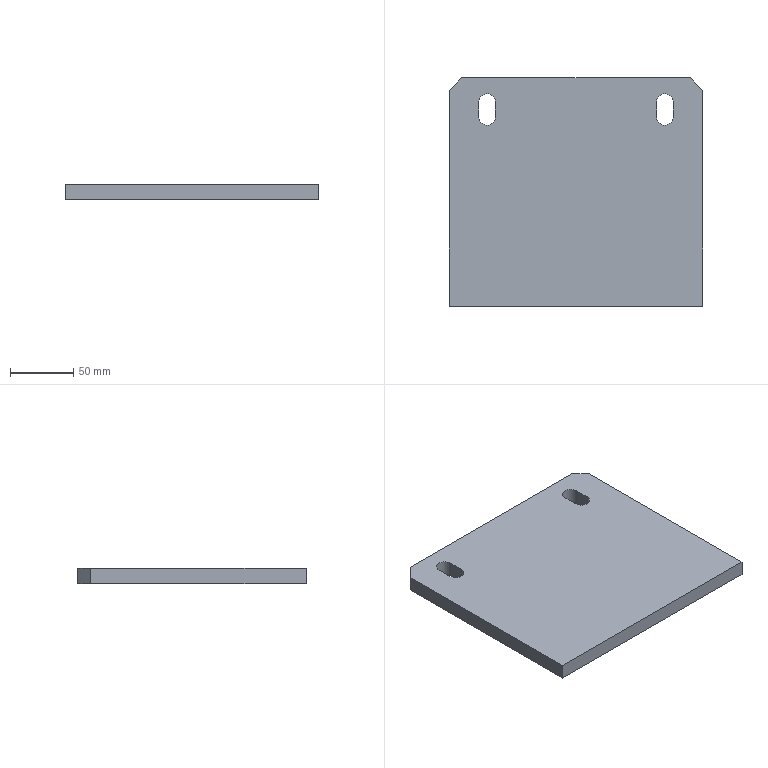Part | SolidWorks | features Chamfer 1, Extrusion 1, ICE 1 | 1 solid | 16 faces | box 200 x 180 x 12 mm | volume 423870 mm3 | plane 12 | cylinder 4 | commonest cylinder face diameters 13 x4
STEP:
#1=CARTESIAN_POINT('',(100.,-90.,0.));
#2=VERTEX_POINT('',#1);
#3=CARTESIAN_POINT('',(-100.,-90.,0.));
#4=VERTEX_POINT('',#3);
#5=CARTESIAN_POINT('',(100.,-90.,0.));
#6=DIRECTION('',(-1.,0.,0.));
#7=VECTOR('',#6,1000.);
#8=LINE('',#5,#7);
#9=EDGE_CURVE('',#2,#4,#8,.T.);
#10=ORIENTED_EDGE('',*,*,#9,.F.);
#11=CARTESIAN_POINT('',(100.,-90.,12.));
#12=VERTEX_POINT('',#11);
#13=CARTESIAN_POINT('',(100.,-90.,12.));
#14=DIRECTION('',(0.,0.,-1.));
#15=VECTOR('',#14,1000.);
#16=LINE('',#13,#15);
#17=EDGE_CURVE('',#12,#2,#16,.T.);
#18=ORIENTED_EDGE('',*,*,#17,.F.);
#19=CARTESIAN_POINT('',(-100.,-90.,12.));
#20=VERTEX_POINT('',#19);
#21=CARTESIAN_POINT('',(100.,-90.,12.));
#22=DIRECTION('',(-1.,0.,0.));
#23=VECTOR('',#22,1000.);
#24=LINE('',#21,#23);
#25=EDGE_CURVE('',#12,#20,#24,.T.);
#26=ORIENTED_EDGE('',*,*,#25,.T.);
#27=CARTESIAN_POINT('',(-100.,-90.,12.));
#28=DIRECTION('',(0.,0.,-1.));
#29=VECTOR('',#28,1000.);
#30=LINE('',#27,#29);
#31=EDGE_CURVE('',#20,#4,#30,.T.);
#32=ORIENTED_EDGE('',*,*,#31,.T.);
#33=EDGE_LOOP('',(#10,#18,#26,#32));
#34=FACE_OUTER_BOUND('',#33,.T.);
#35=CARTESIAN_POINT('',(100.,-90.,12.));
#36=DIRECTION('',(0.,-1.,0.));
#37=DIRECTION('',(1.,0.,0.));
#38=AXIS2_PLACEMENT_3D('',#35,#36,#37);
#39=PLANE('',#38);
#40=ADVANCED_FACE('',(#34),#39,.T.);
#41=CARTESIAN_POINT('',(100.,80.,0.));
#42=VERTEX_POINT('',#41);
#43=CARTESIAN_POINT('',(100.,90.,0.));
#44=DIRECTION('',(0.,-1.,0.));
#45=VECTOR('',#44,1000.);
#46=LINE('',#43,#45);
#47=EDGE_CURVE('',#42,#2,#46,.T.);
#48=ORIENTED_EDGE('',*,*,#47,.F.);
#49=CARTESIAN_POINT('',(100.,80.,12.));
#50=VERTEX_POINT('',#49);
#51=CARTESIAN_POINT('',(100.,80.,12.));
#52=DIRECTION('',(0.,0.,1.));
#53=VECTOR('',#52,1000.);
#54=LINE('',#51,#53);
#55=EDGE_CURVE('',#42,#50,#54,.T.);
#56=ORIENTED_EDGE('',*,*,#55,.T.);
#57=CARTESIAN_POINT('',(100.,90.,12.));
#58=DIRECTION('',(0.,-1.,0.));
#59=VECTOR('',#58,1000.);
#60=LINE('',#57,#59);
#61=EDGE_CURVE('',#50,#12,#60,.T.);
#62=ORIENTED_EDGE('',*,*,#61,.T.);
#63=ORIENTED_EDGE('',*,*,#17,.T.);
#64=EDGE_LOOP('',(#48,#56,#62,#63));
#65=FACE_OUTER_BOUND('',#64,.T.);
#66=CARTESIAN_POINT('',(100.,90.,12.));
#67=DIRECTION('',(1.,0.,0.));
#68=DIRECTION('',(0.,0.,-1.));
#69=AXIS2_PLACEMENT_3D('',#66,#67,#68);
#70=PLANE('',#69);
#71=ADVANCED_FACE('',(#65),#70,.T.);
#72=CARTESIAN_POINT('',(90.,90.,0.));
#73=VERTEX_POINT('',#72);
#74=CARTESIAN_POINT('',(-90.,90.,0.));
#75=VERTEX_POINT('',#74);
#76=CARTESIAN_POINT('',(100.,90.,0.));
#77=DIRECTION('',(-1.,0.,0.));
#78=VECTOR('',#77,1000.);
#79=LINE('',#76,#78);
#80=EDGE_CURVE('',#73,#75,#79,.T.);
#81=ORIENTED_EDGE('',*,*,#80,.T.);
#82=CARTESIAN_POINT('',(-90.,90.,12.));
#83=VERTEX_POINT('',#82);
#84=CARTESIAN_POINT('',(-90.,90.,12.));
#85=DIRECTION('',(0.,0.,1.));
#86=VECTOR('',#85,1000.);
#87=LINE('',#84,#86);
#88=EDGE_CURVE('',#75,#83,#87,.T.);
#89=ORIENTED_EDGE('',*,*,#88,.T.);
#90=CARTESIAN_POINT('',(90.,90.,12.));
#91=VERTEX_POINT('',#90);
#92=CARTESIAN_POINT('',(100.,90.,12.));
#93=DIRECTION('',(-1.,0.,0.));
#94=VECTOR('',#93,1000.);
#95=LINE('',#92,#94);
#96=EDGE_CURVE('',#91,#83,#95,.T.);
#97=ORIENTED_EDGE('',*,*,#96,.F.);
#98=CARTESIAN_POINT('',(90.,90.,0.));
#99=DIRECTION('',(0.,0.,-1.));
#100=VECTOR('',#99,1000.);
#101=LINE('',#98,#100);
#102=EDGE_CURVE('',#91,#73,#101,.T.);
#103=ORIENTED_EDGE('',*,*,#102,.T.);
#104=EDGE_LOOP('',(#81,#89,#97,#103));
#105=FACE_OUTER_BOUND('',#104,.T.);
#106=CARTESIAN_POINT('',(100.,90.,12.));
#107=DIRECTION('',(0.,-1.,0.));
#108=DIRECTION('',(1.,0.,0.));
#109=AXIS2_PLACEMENT_3D('',#106,#107,#108);
#110=PLANE('',#109);
#111=ADVANCED_FACE('',(#105),#110,.F.);
#112=CARTESIAN_POINT('',(-100.,80.,12.));
#113=VERTEX_POINT('',#112);
#114=CARTESIAN_POINT('',(-100.,90.,12.));
#115=DIRECTION('',(0.,-1.,0.));
#116=VECTOR('',#115,1000.);
#117=LINE('',#114,#116);
#118=EDGE_CURVE('',#113,#20,#117,.T.);
#119=ORIENTED_EDGE('',*,*,#118,.F.);
#120=CARTESIAN_POINT('',(-100.,80.,0.));
#121=VERTEX_POINT('',#120);
#122=CARTESIAN_POINT('',(-100.,80.,12.));
#123=DIRECTION('',(0.,0.,-1.));
#124=VECTOR('',#123,1000.);
#125=LINE('',#122,#124);
#126=EDGE_CURVE('',#113,#121,#125,.T.);
#127=ORIENTED_EDGE('',*,*,#126,.T.);
#128=CARTESIAN_POINT('',(-100.,90.,0.));
#129=DIRECTION('',(0.,-1.,0.));
#130=VECTOR('',#129,1000.);
#131=LINE('',#128,#130);
#132=EDGE_CURVE('',#121,#4,#131,.T.);
#133=ORIENTED_EDGE('',*,*,#132,.T.);
#134=ORIENTED_EDGE('',*,*,#31,.F.);
#135=EDGE_LOOP('',(#119,#127,#133,#134));
#136=FACE_OUTER_BOUND('',#135,.T.);
#137=CARTESIAN_POINT('',(-100.,90.,12.));
#138=DIRECTION('',(1.,0.,0.));
#139=DIRECTION('',(0.,1.,0.));
#140=AXIS2_PLACEMENT_3D('',#137,#138,#139);
#141=PLANE('',#140);
#142=ADVANCED_FACE('',(#136),#141,.F.);
#143=CARTESIAN_POINT('',(-63.5,71.,12.));
#144=VERTEX_POINT('',#143);
#145=CARTESIAN_POINT('',(-76.5,71.,12.));
#146=VERTEX_POINT('',#145);
#147=CARTESIAN_POINT('',(-70.,71.,12.));
#148=DIRECTION('',(0.,0.,1.));
#149=DIRECTION('',(1.,0.,0.));
#150=AXIS2_PLACEMENT_3D('',#147,#148,#149);
#151=CIRCLE('',#150,6.5);
#152=EDGE_CURVE('',#144,#146,#151,.T.);
#153=ORIENTED_EDGE('',*,*,#152,.F.);
#154=CARTESIAN_POINT('',(-63.5,59.,12.));
#155=VERTEX_POINT('',#154);
#156=CARTESIAN_POINT('',(-63.5,71.,12.));
#157=DIRECTION('',(0.,1.,0.));
#158=VECTOR('',#157,1000.);
#159=LINE('',#156,#158);
#160=EDGE_CURVE('',#155,#144,#159,.T.);
#161=ORIENTED_EDGE('',*,*,#160,.F.);
#162=CARTESIAN_POINT('',(-76.5,59.,12.));
#163=VERTEX_POINT('',#162);
#164=CARTESIAN_POINT('',(-70.,59.,12.));
#165=DIRECTION('',(0.,0.,1.));
#166=DIRECTION('',(1.,0.,0.));
#167=AXIS2_PLACEMENT_3D('',#164,#165,#166);
#168=CIRCLE('',#167,6.5);
#169=EDGE_CURVE('',#163,#155,#168,.T.);
#170=ORIENTED_EDGE('',*,*,#169,.F.);
#171=CARTESIAN_POINT('',(-76.5,71.,12.));
#172=DIRECTION('',(0.,-1.,0.));
#173=VECTOR('',#172,1000.);
#174=LINE('',#171,#173);
#175=EDGE_CURVE('',#146,#163,#174,.T.);
#176=ORIENTED_EDGE('',*,*,#175,.F.);
#177=EDGE_LOOP('',(#153,#161,#170,#176));
#178=FACE_BOUND('',#177,.T.);
#179=CARTESIAN_POINT('',(76.5,71.,12.));
#180=VERTEX_POINT('',#179);
#181=CARTESIAN_POINT('',(63.5,71.,12.));
#182=VERTEX_POINT('',#181);
#183=CARTESIAN_POINT('',(70.,71.,12.));
#184=DIRECTION('',(0.,0.,1.));
#185=DIRECTION('',(1.,0.,0.));
#186=AXIS2_PLACEMENT_3D('',#183,#184,#185);
#187=CIRCLE('',#186,6.5);
#188=EDGE_CURVE('',#180,#182,#187,.T.);
#189=ORIENTED_EDGE('',*,*,#188,.F.);
#190=CARTESIAN_POINT('',(76.5,59.,12.));
#191=VERTEX_POINT('',#190);
#192=CARTESIAN_POINT('',(76.5,71.,12.));
#193=DIRECTION('',(0.,1.,0.));
#194=VECTOR('',#193,1000.);
#195=LINE('',#192,#194);
#196=EDGE_CURVE('',#191,#180,#195,.T.);
#197=ORIENTED_EDGE('',*,*,#196,.F.);
#198=CARTESIAN_POINT('',(63.5,59.,12.));
#199=VERTEX_POINT('',#198);
#200=CARTESIAN_POINT('',(70.,59.,12.));
#201=DIRECTION('',(0.,0.,1.));
#202=DIRECTION('',(1.,0.,0.));
#203=AXIS2_PLACEMENT_3D('',#200,#201,#202);
#204=CIRCLE('',#203,6.5);
#205=EDGE_CURVE('',#199,#191,#204,.T.);
#206=ORIENTED_EDGE('',*,*,#205,.F.);
#207=CARTESIAN_POINT('',(63.5,71.,12.));
#208=DIRECTION('',(0.,-1.,0.));
#209=VECTOR('',#208,1000.);
#210=LINE('',#207,#209);
#211=EDGE_CURVE('',#182,#199,#210,.T.);
#212=ORIENTED_EDGE('',*,*,#211,.F.);
#213=EDGE_LOOP('',(#189,#197,#206,#212));
#214=FACE_BOUND('',#213,.T.);
#215=ORIENTED_EDGE('',*,*,#96,.T.);
#216=CARTESIAN_POINT('',(-90.,90.,12.));
#217=DIRECTION('',(-0.7071,-0.7071,0.));
#218=VECTOR('',#217,1000.);
#219=LINE('',#216,#218);
#220=EDGE_CURVE('',#83,#113,#219,.T.);
#221=ORIENTED_EDGE('',*,*,#220,.T.);
#222=ORIENTED_EDGE('',*,*,#118,.T.);
#223=ORIENTED_EDGE('',*,*,#25,.F.);
#224=ORIENTED_EDGE('',*,*,#61,.F.);
#225=CARTESIAN_POINT('',(90.,90.,12.));
#226=DIRECTION('',(-0.7071,0.7071,0.));
#227=VECTOR('',#226,1000.);
#228=LINE('',#225,#227);
#229=EDGE_CURVE('',#50,#91,#228,.T.);
#230=ORIENTED_EDGE('',*,*,#229,.T.);
#231=EDGE_LOOP('',(#215,#221,#222,#223,#224,#230));
#232=FACE_OUTER_BOUND('',#231,.T.);
#233=CARTESIAN_POINT('',(0.,0.,12.));
#234=DIRECTION('',(0.,0.,1.));
#235=DIRECTION('',(1.,0.,0.));
#236=AXIS2_PLACEMENT_3D('',#233,#234,#235);
#237=PLANE('',#236);
#238=ADVANCED_FACE('',(#178,#214,#232),#237,.T.);
#239=CARTESIAN_POINT('',(-63.5,59.,0.));
#240=VERTEX_POINT('',#239);
#241=CARTESIAN_POINT('',(-63.5,71.,0.));
#242=VERTEX_POINT('',#241);
#243=CARTESIAN_POINT('',(-63.5,71.,0.));
#244=DIRECTION('',(0.,1.,0.));
#245=VECTOR('',#244,1000.);
#246=LINE('',#243,#245);
#247=EDGE_CURVE('',#240,#242,#246,.T.);
#248=ORIENTED_EDGE('',*,*,#247,.T.);
#249=CARTESIAN_POINT('',(-76.5,71.,0.));
#250=VERTEX_POINT('',#249);
#251=CARTESIAN_POINT('',(-70.,71.,0.));
#252=DIRECTION('',(0.,0.,1.));
#253=DIRECTION('',(1.,0.,0.));
#254=AXIS2_PLACEMENT_3D('',#251,#252,#253);
#255=CIRCLE('',#254,6.5);
#256=EDGE_CURVE('',#242,#250,#255,.T.);
#257=ORIENTED_EDGE('',*,*,#256,.T.);
#258=CARTESIAN_POINT('',(-76.5,59.,0.));
#259=VERTEX_POINT('',#258);
#260=CARTESIAN_POINT('',(-76.5,71.,0.));
#261=DIRECTION('',(0.,-1.,0.));
#262=VECTOR('',#261,1000.);
#263=LINE('',#260,#262);
#264=EDGE_CURVE('',#250,#259,#263,.T.);
#265=ORIENTED_EDGE('',*,*,#264,.T.);
#266=CARTESIAN_POINT('',(-70.,59.,0.));
#267=DIRECTION('',(0.,0.,1.));
#268=DIRECTION('',(1.,0.,0.));
#269=AXIS2_PLACEMENT_3D('',#266,#267,#268);
#270=CIRCLE('',#269,6.5);
#271=EDGE_CURVE('',#259,#240,#270,.T.);
#272=ORIENTED_EDGE('',*,*,#271,.T.);
#273=EDGE_LOOP('',(#248,#257,#265,#272));
#274=FACE_BOUND('',#273,.T.);
#275=CARTESIAN_POINT('',(76.5,59.,0.));
#276=VERTEX_POINT('',#275);
#277=CARTESIAN_POINT('',(76.5,71.,0.));
#278=VERTEX_POINT('',#277);
#279=CARTESIAN_POINT('',(76.5,71.,0.));
#280=DIRECTION('',(0.,1.,0.));
#281=VECTOR('',#280,1000.);
#282=LINE('',#279,#281);
#283=EDGE_CURVE('',#276,#278,#282,.T.);
#284=ORIENTED_EDGE('',*,*,#283,.T.);
#285=CARTESIAN_POINT('',(63.5,71.,0.));
#286=VERTEX_POINT('',#285);
#287=CARTESIAN_POINT('',(70.,71.,0.));
#288=DIRECTION('',(0.,0.,1.));
#289=DIRECTION('',(1.,0.,0.));
#290=AXIS2_PLACEMENT_3D('',#287,#288,#289);
#291=CIRCLE('',#290,6.5);
#292=EDGE_CURVE('',#278,#286,#291,.T.);
#293=ORIENTED_EDGE('',*,*,#292,.T.);
#294=CARTESIAN_POINT('',(63.5,59.,0.));
#295=VERTEX_POINT('',#294);
#296=CARTESIAN_POINT('',(63.5,71.,0.));
#297=DIRECTION('',(0.,-1.,0.));
#298=VECTOR('',#297,1000.);
#299=LINE('',#296,#298);
#300=EDGE_CURVE('',#286,#295,#299,.T.);
#301=ORIENTED_EDGE('',*,*,#300,.T.);
#302=CARTESIAN_POINT('',(70.,59.,0.));
#303=DIRECTION('',(0.,0.,1.));
#304=DIRECTION('',(1.,0.,0.));
#305=AXIS2_PLACEMENT_3D('',#302,#303,#304);
#306=CIRCLE('',#305,6.5);
#307=EDGE_CURVE('',#295,#276,#306,.T.);
#308=ORIENTED_EDGE('',*,*,#307,.T.);
#309=EDGE_LOOP('',(#284,#293,#301,#308));
#310=FACE_BOUND('',#309,.T.);
#311=ORIENTED_EDGE('',*,*,#132,.F.);
#312=CARTESIAN_POINT('',(-100.,80.,0.));
#313=DIRECTION('',(0.7071,0.7071,0.));
#314=VECTOR('',#313,1000.);
#315=LINE('',#312,#314);
#316=EDGE_CURVE('',#121,#75,#315,.T.);
#317=ORIENTED_EDGE('',*,*,#316,.T.);
#318=ORIENTED_EDGE('',*,*,#80,.F.);
#319=CARTESIAN_POINT('',(90.,90.,0.));
#320=DIRECTION('',(0.7071,-0.7071,0.));
#321=VECTOR('',#320,1000.);
#322=LINE('',#319,#321);
#323=EDGE_CURVE('',#73,#42,#322,.T.);
#324=ORIENTED_EDGE('',*,*,#323,.T.);
#325=ORIENTED_EDGE('',*,*,#47,.T.);
#326=ORIENTED_EDGE('',*,*,#9,.T.);
#327=EDGE_LOOP('',(#311,#317,#318,#324,#325,#326));
#328=FACE_OUTER_BOUND('',#327,.T.);
#329=CARTESIAN_POINT('',(0.,0.,0.));
#330=DIRECTION('',(0.,0.,1.));
#331=DIRECTION('',(1.,0.,0.));
#332=AXIS2_PLACEMENT_3D('',#329,#330,#331);
#333=PLANE('',#332);
#334=ADVANCED_FACE('',(#274,#310,#328),#333,.F.);
#335=ORIENTED_EDGE('',*,*,#220,.F.);
#336=ORIENTED_EDGE('',*,*,#88,.F.);
#337=ORIENTED_EDGE('',*,*,#316,.F.);
#338=ORIENTED_EDGE('',*,*,#126,.F.);
#339=EDGE_LOOP('',(#335,#336,#337,#338));
#340=FACE_OUTER_BOUND('',#339,.T.);
#341=CARTESIAN_POINT('',(-100.,80.,12.));
#342=DIRECTION('',(0.7071,-0.7071,0.));
#343=DIRECTION('',(0.,0.,-1.));
#344=AXIS2_PLACEMENT_3D('',#341,#342,#343);
#345=PLANE('',#344);
#346=ADVANCED_FACE('',(#340),#345,.F.);
#347=ORIENTED_EDGE('',*,*,#229,.F.);
#348=ORIENTED_EDGE('',*,*,#55,.F.);
#349=ORIENTED_EDGE('',*,*,#323,.F.);
#350=ORIENTED_EDGE('',*,*,#102,.F.);
#351=EDGE_LOOP('',(#347,#348,#349,#350));
#352=FACE_OUTER_BOUND('',#351,.T.);
#353=CARTESIAN_POINT('',(90.,90.,12.));
#354=DIRECTION('',(0.7071,0.7071,0.));
#355=DIRECTION('',(0.,0.,1.));
#356=AXIS2_PLACEMENT_3D('',#353,#354,#355);
#357=PLANE('',#356);
#358=ADVANCED_FACE('',(#352),#357,.T.);
#359=ORIENTED_EDGE('',*,*,#188,.T.);
#360=CARTESIAN_POINT('',(63.5,71.,0.));
#361=DIRECTION('',(0.,0.,1.));
#362=VECTOR('',#361,1000.);
#363=LINE('',#360,#362);
#364=EDGE_CURVE('',#286,#182,#363,.T.);
#365=ORIENTED_EDGE('',*,*,#364,.F.);
#366=ORIENTED_EDGE('',*,*,#292,.F.);
#367=CARTESIAN_POINT('',(76.5,71.,0.));
#368=DIRECTION('',(0.,0.,1.));
#369=VECTOR('',#368,1000.);
#370=LINE('',#367,#369);
#371=EDGE_CURVE('',#278,#180,#370,.T.);
#372=ORIENTED_EDGE('',*,*,#371,.T.);
#373=EDGE_LOOP('',(#359,#365,#366,#372));
#374=FACE_OUTER_BOUND('',#373,.T.);
#375=CARTESIAN_POINT('',(70.,71.,0.));
#376=DIRECTION('',(0.,0.,1.));
#377=DIRECTION('',(1.,0.,0.));
#378=AXIS2_PLACEMENT_3D('',#375,#376,#377);
#379=CYLINDRICAL_SURFACE('',#378,6.5);
#380=ADVANCED_FACE('',(#374),#379,.F.);
#381=ORIENTED_EDGE('',*,*,#196,.T.);
#382=ORIENTED_EDGE('',*,*,#371,.F.);
#383=ORIENTED_EDGE('',*,*,#283,.F.);
#384=CARTESIAN_POINT('',(76.5,59.,0.));
#385=DIRECTION('',(0.,0.,1.));
#386=VECTOR('',#385,1000.);
#387=LINE('',#384,#386);
#388=EDGE_CURVE('',#276,#191,#387,.T.);
#389=ORIENTED_EDGE('',*,*,#388,.T.);
#390=EDGE_LOOP('',(#381,#382,#383,#389));
#391=FACE_OUTER_BOUND('',#390,.T.);
#392=CARTESIAN_POINT('',(76.5,71.,0.));
#393=DIRECTION('',(1.,0.,0.));
#394=DIRECTION('',(0.,0.,-1.));
#395=AXIS2_PLACEMENT_3D('',#392,#393,#394);
#396=PLANE('',#395);
#397=ADVANCED_FACE('',(#391),#396,.F.);
#398=ORIENTED_EDGE('',*,*,#205,.T.);
#399=ORIENTED_EDGE('',*,*,#388,.F.);
#400=ORIENTED_EDGE('',*,*,#307,.F.);
#401=CARTESIAN_POINT('',(63.5,59.,0.));
#402=DIRECTION('',(0.,0.,1.));
#403=VECTOR('',#402,1000.);
#404=LINE('',#401,#403);
#405=EDGE_CURVE('',#295,#199,#404,.T.);
#406=ORIENTED_EDGE('',*,*,#405,.T.);
#407=EDGE_LOOP('',(#398,#399,#400,#406));
#408=FACE_OUTER_BOUND('',#407,.T.);
#409=CARTESIAN_POINT('',(70.,59.,0.));
#410=DIRECTION('',(0.,0.,1.));
#411=DIRECTION('',(1.,0.,0.));
#412=AXIS2_PLACEMENT_3D('',#409,#410,#411);
#413=CYLINDRICAL_SURFACE('',#412,6.5);
#414=ADVANCED_FACE('',(#408),#413,.F.);
#415=ORIENTED_EDGE('',*,*,#211,.T.);
#416=ORIENTED_EDGE('',*,*,#405,.F.);
#417=ORIENTED_EDGE('',*,*,#300,.F.);
#418=ORIENTED_EDGE('',*,*,#364,.T.);
#419=EDGE_LOOP('',(#415,#416,#417,#418));
#420=FACE_OUTER_BOUND('',#419,.T.);
#421=CARTESIAN_POINT('',(63.5,71.,0.));
#422=DIRECTION('',(-1.,0.,0.));
#423=DIRECTION('',(0.,0.,1.));
#424=AXIS2_PLACEMENT_3D('',#421,#422,#423);
#425=PLANE('',#424);
#426=ADVANCED_FACE('',(#420),#425,.F.);
#427=ORIENTED_EDGE('',*,*,#152,.T.);
#428=CARTESIAN_POINT('',(-76.5,71.,0.));
#429=DIRECTION('',(0.,0.,1.));
#430=VECTOR('',#429,1000.);
#431=LINE('',#428,#430);
#432=EDGE_CURVE('',#250,#146,#431,.T.);
#433=ORIENTED_EDGE('',*,*,#432,.F.);
#434=ORIENTED_EDGE('',*,*,#256,.F.);
#435=CARTESIAN_POINT('',(-63.5,71.,0.));
#436=DIRECTION('',(0.,0.,1.));
#437=VECTOR('',#436,1000.);
#438=LINE('',#435,#437);
#439=EDGE_CURVE('',#242,#144,#438,.T.);
#440=ORIENTED_EDGE('',*,*,#439,.T.);
#441=EDGE_LOOP('',(#427,#433,#434,#440));
#442=FACE_OUTER_BOUND('',#441,.T.);
#443=CARTESIAN_POINT('',(-70.,71.,0.));
#444=DIRECTION('',(0.,0.,1.));
#445=DIRECTION('',(1.,0.,0.));
#446=AXIS2_PLACEMENT_3D('',#443,#444,#445);
#447=CYLINDRICAL_SURFACE('',#446,6.5);
#448=ADVANCED_FACE('',(#442),#447,.F.);
#449=ORIENTED_EDGE('',*,*,#160,.T.);
#450=ORIENTED_EDGE('',*,*,#439,.F.);
#451=ORIENTED_EDGE('',*,*,#247,.F.);
#452=CARTESIAN_POINT('',(-63.5,59.,0.));
#453=DIRECTION('',(0.,0.,1.));
#454=VECTOR('',#453,1000.);
#455=LINE('',#452,#454);
#456=EDGE_CURVE('',#240,#155,#455,.T.);
#457=ORIENTED_EDGE('',*,*,#456,.T.);
#458=EDGE_LOOP('',(#449,#450,#451,#457));
#459=FACE_OUTER_BOUND('',#458,.T.);
#460=CARTESIAN_POINT('',(-63.5,71.,0.));
#461=DIRECTION('',(1.,0.,0.));
#462=DIRECTION('',(0.,0.,-1.));
#463=AXIS2_PLACEMENT_3D('',#460,#461,#462);
#464=PLANE('',#463);
#465=ADVANCED_FACE('',(#459),#464,.F.);
#466=ORIENTED_EDGE('',*,*,#169,.T.);
#467=ORIENTED_EDGE('',*,*,#456,.F.);
#468=ORIENTED_EDGE('',*,*,#271,.F.);
#469=CARTESIAN_POINT('',(-76.5,59.,0.));
#470=DIRECTION('',(0.,0.,1.));
#471=VECTOR('',#470,1000.);
#472=LINE('',#469,#471);
#473=EDGE_CURVE('',#259,#163,#472,.T.);
#474=ORIENTED_EDGE('',*,*,#473,.T.);
#475=EDGE_LOOP('',(#466,#467,#468,#474));
#476=FACE_OUTER_BOUND('',#475,.T.);
#477=CARTESIAN_POINT('',(-70.,59.,0.));
#478=DIRECTION('',(0.,0.,1.));
#479=DIRECTION('',(1.,0.,0.));
#480=AXIS2_PLACEMENT_3D('',#477,#478,#479);
#481=CYLINDRICAL_SURFACE('',#480,6.5);
#482=ADVANCED_FACE('',(#476),#481,.F.);
#483=ORIENTED_EDGE('',*,*,#175,.T.);
#484=ORIENTED_EDGE('',*,*,#473,.F.);
#485=ORIENTED_EDGE('',*,*,#264,.F.);
#486=ORIENTED_EDGE('',*,*,#432,.T.);
#487=EDGE_LOOP('',(#483,#484,#485,#486));
#488=FACE_OUTER_BOUND('',#487,.T.);
#489=CARTESIAN_POINT('',(-76.5,71.,0.));
#490=DIRECTION('',(-1.,0.,0.));
#491=DIRECTION('',(0.,0.,1.));
#492=AXIS2_PLACEMENT_3D('',#489,#490,#491);
#493=PLANE('',#492);
#494=ADVANCED_FACE('',(#488),#493,.F.);
#495=CLOSED_SHELL('',(#40,#71,#111,#142,#238,#334,#346,#358,#380,#397,#414,#426,#448,#465,#482,#494));
#496=MANIFOLD_SOLID_BREP('',#495);
#497=CARTESIAN_POINT('',(0.,0.,0.));
#498=DIRECTION('',(0.,0.,1.));
#499=DIRECTION('',(1.,0.,0.));
#500=AXIS2_PLACEMENT_3D('',#497,#498,#499);
#501=(LENGTH_UNIT()NAMED_UNIT(*)SI_UNIT(.MILLI.,.METRE.));
#502=UNCERTAINTY_MEASURE_WITH_UNIT(LENGTH_MEASURE(0.00001),#501,'','');
#503=(NAMED_UNIT(*)PLANE_ANGLE_UNIT()SI_UNIT($,.RADIAN.));
#504=(NAMED_UNIT(*)SI_UNIT($,.STERADIAN.)SOLID_ANGLE_UNIT());
#505=(GEOMETRIC_REPRESENTATION_CONTEXT(3)GLOBAL_UNCERTAINTY_ASSIGNED_CONTEXT((#502))GLOBAL_UNIT_ASSIGNED_CONTEXT((#501,#503,#504))REPRESENTATION_CONTEXT('',''));
#506=ADVANCED_BREP_SHAPE_REPRESENTATION('',(#496,#500),#505);